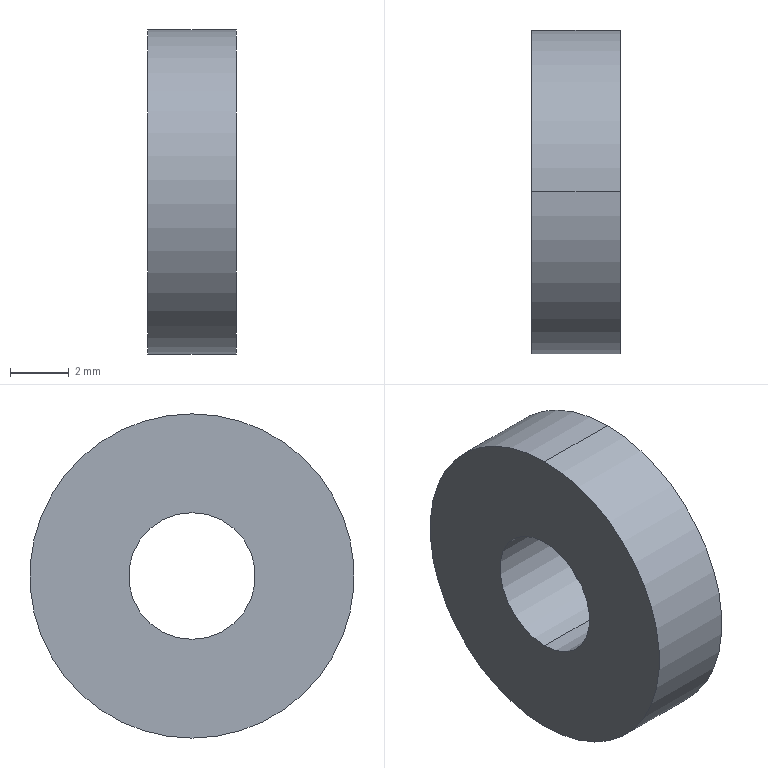Part | STEP file | 11-FJTM4_0_7_413part211 | 1 solid | 6 faces | box 3 x 11 x 11 mm | volume 241.533 mm3 | cylinder 4 | plane 2 | commonest cylinder face diameters 4.3 x2 11 x2
STEP:
#1=CARTESIAN_POINT('',(3.,0.,5.5));
#2=VERTEX_POINT('',#1);
#3=CARTESIAN_POINT('',(3.,0.,-5.5));
#4=VERTEX_POINT('',#3);
#5=CARTESIAN_POINT('',(3.,0.,0.));
#6=DIRECTION('',(-1.,0.,0.));
#7=DIRECTION('',(0.,0.,1.));
#8=AXIS2_PLACEMENT_3D('',#5,#6,#7);
#9=CIRCLE('',#8,5.5);
#10=EDGE_CURVE('',#2,#4,#9,.T.);
#11=ORIENTED_EDGE('',*,*,#10,.T.);
#12=CARTESIAN_POINT('',(0.,0.,-5.5));
#13=VERTEX_POINT('',#12);
#14=CARTESIAN_POINT('',(3.,0.,-5.5));
#15=DIRECTION('',(-1.,0.,0.));
#16=VECTOR('',#15,1000.);
#17=LINE('',#14,#16);
#18=EDGE_CURVE('',#4,#13,#17,.T.);
#19=ORIENTED_EDGE('',*,*,#18,.T.);
#20=CARTESIAN_POINT('',(0.,0.,5.5));
#21=VERTEX_POINT('',#20);
#22=CARTESIAN_POINT('',(0.,0.,0.));
#23=DIRECTION('',(-1.,0.,0.));
#24=DIRECTION('',(0.,0.,1.));
#25=AXIS2_PLACEMENT_3D('',#22,#23,#24);
#26=CIRCLE('',#25,5.5);
#27=EDGE_CURVE('',#21,#13,#26,.T.);
#28=ORIENTED_EDGE('',*,*,#27,.F.);
#29=CARTESIAN_POINT('',(3.,0.,5.5));
#30=DIRECTION('',(-1.,0.,0.));
#31=VECTOR('',#30,1000.);
#32=LINE('',#29,#31);
#33=EDGE_CURVE('',#2,#21,#32,.T.);
#34=ORIENTED_EDGE('',*,*,#33,.F.);
#35=EDGE_LOOP('',(#11,#19,#28,#34));
#36=FACE_OUTER_BOUND('',#35,.T.);
#37=CARTESIAN_POINT('',(3.,0.,0.));
#38=DIRECTION('',(-1.,0.,0.));
#39=DIRECTION('',(0.,0.,1.));
#40=AXIS2_PLACEMENT_3D('',#37,#38,#39);
#41=CYLINDRICAL_SURFACE('',#40,5.5);
#42=ADVANCED_FACE('',(#36),#41,.T.);
#43=CARTESIAN_POINT('',(3.,0.,-2.15));
#44=VERTEX_POINT('',#43);
#45=CARTESIAN_POINT('',(3.,0.,2.15));
#46=VERTEX_POINT('',#45);
#47=CARTESIAN_POINT('',(3.,0.,0.));
#48=DIRECTION('',(-1.,0.,0.));
#49=DIRECTION('',(0.,0.,1.));
#50=AXIS2_PLACEMENT_3D('',#47,#48,#49);
#51=CIRCLE('',#50,2.15);
#52=EDGE_CURVE('',#44,#46,#51,.T.);
#53=ORIENTED_EDGE('',*,*,#52,.F.);
#54=CARTESIAN_POINT('',(0.,0.,-2.15));
#55=VERTEX_POINT('',#54);
#56=CARTESIAN_POINT('',(3.,0.,-2.15));
#57=DIRECTION('',(-1.,0.,0.));
#58=VECTOR('',#57,1000.);
#59=LINE('',#56,#58);
#60=EDGE_CURVE('',#44,#55,#59,.T.);
#61=ORIENTED_EDGE('',*,*,#60,.T.);
#62=CARTESIAN_POINT('',(0.,0.,2.15));
#63=VERTEX_POINT('',#62);
#64=CARTESIAN_POINT('',(0.,0.,0.));
#65=DIRECTION('',(-1.,0.,0.));
#66=DIRECTION('',(0.,0.,1.));
#67=AXIS2_PLACEMENT_3D('',#64,#65,#66);
#68=CIRCLE('',#67,2.15);
#69=EDGE_CURVE('',#55,#63,#68,.T.);
#70=ORIENTED_EDGE('',*,*,#69,.T.);
#71=CARTESIAN_POINT('',(3.,0.,2.15));
#72=DIRECTION('',(-1.,0.,0.));
#73=VECTOR('',#72,1000.);
#74=LINE('',#71,#73);
#75=EDGE_CURVE('',#46,#63,#74,.T.);
#76=ORIENTED_EDGE('',*,*,#75,.F.);
#77=EDGE_LOOP('',(#53,#61,#70,#76));
#78=FACE_OUTER_BOUND('',#77,.T.);
#79=CARTESIAN_POINT('',(3.,0.,0.));
#80=DIRECTION('',(-1.,0.,0.));
#81=DIRECTION('',(0.,0.,1.));
#82=AXIS2_PLACEMENT_3D('',#79,#80,#81);
#83=CYLINDRICAL_SURFACE('',#82,2.15);
#84=ADVANCED_FACE('',(#78),#83,.F.);
#85=CARTESIAN_POINT('',(0.,0.,0.));
#86=DIRECTION('',(-1.,0.,0.));
#87=DIRECTION('',(0.,0.,1.));
#88=AXIS2_PLACEMENT_3D('',#85,#86,#87);
#89=CIRCLE('',#88,2.15);
#90=EDGE_CURVE('',#63,#55,#89,.T.);
#91=ORIENTED_EDGE('',*,*,#90,.F.);
#92=ORIENTED_EDGE('',*,*,#69,.F.);
#93=EDGE_LOOP('',(#91,#92));
#94=FACE_BOUND('',#93,.T.);
#95=ORIENTED_EDGE('',*,*,#27,.T.);
#96=CARTESIAN_POINT('',(0.,0.,0.));
#97=DIRECTION('',(-1.,0.,0.));
#98=DIRECTION('',(0.,0.,1.));
#99=AXIS2_PLACEMENT_3D('',#96,#97,#98);
#100=CIRCLE('',#99,5.5);
#101=EDGE_CURVE('',#13,#21,#100,.T.);
#102=ORIENTED_EDGE('',*,*,#101,.T.);
#103=EDGE_LOOP('',(#95,#102));
#104=FACE_OUTER_BOUND('',#103,.T.);
#105=CARTESIAN_POINT('',(0.,5.5,0.));
#106=DIRECTION('',(1.,0.,0.));
#107=DIRECTION('',(0.,0.,-1.));
#108=AXIS2_PLACEMENT_3D('',#105,#106,#107);
#109=PLANE('',#108);
#110=ADVANCED_FACE('',(#94,#104),#109,.F.);
#111=ORIENTED_EDGE('',*,*,#60,.F.);
#112=CARTESIAN_POINT('',(3.,0.,0.));
#113=DIRECTION('',(-1.,0.,0.));
#114=DIRECTION('',(0.,0.,1.));
#115=AXIS2_PLACEMENT_3D('',#112,#113,#114);
#116=CIRCLE('',#115,2.15);
#117=EDGE_CURVE('',#46,#44,#116,.T.);
#118=ORIENTED_EDGE('',*,*,#117,.F.);
#119=ORIENTED_EDGE('',*,*,#75,.T.);
#120=ORIENTED_EDGE('',*,*,#90,.T.);
#121=EDGE_LOOP('',(#111,#118,#119,#120));
#122=FACE_OUTER_BOUND('',#121,.T.);
#123=CARTESIAN_POINT('',(3.,0.,0.));
#124=DIRECTION('',(-1.,0.,0.));
#125=DIRECTION('',(0.,0.,1.));
#126=AXIS2_PLACEMENT_3D('',#123,#124,#125);
#127=CYLINDRICAL_SURFACE('',#126,2.15);
#128=ADVANCED_FACE('',(#122),#127,.F.);
#129=ORIENTED_EDGE('',*,*,#10,.F.);
#130=CARTESIAN_POINT('',(3.,0.,0.));
#131=DIRECTION('',(-1.,0.,0.));
#132=DIRECTION('',(0.,0.,1.));
#133=AXIS2_PLACEMENT_3D('',#130,#131,#132);
#134=CIRCLE('',#133,5.5);
#135=EDGE_CURVE('',#4,#2,#134,.T.);
#136=ORIENTED_EDGE('',*,*,#135,.F.);
#137=EDGE_LOOP('',(#129,#136));
#138=FACE_OUTER_BOUND('',#137,.T.);
#139=ORIENTED_EDGE('',*,*,#117,.T.);
#140=ORIENTED_EDGE('',*,*,#52,.T.);
#141=EDGE_LOOP('',(#139,#140));
#142=FACE_BOUND('',#141,.T.);
#143=CARTESIAN_POINT('',(3.,2.15,0.));
#144=DIRECTION('',(-1.,0.,0.));
#145=DIRECTION('',(0.,0.,1.));
#146=AXIS2_PLACEMENT_3D('',#143,#144,#145);
#147=PLANE('',#146);
#148=ADVANCED_FACE('',(#138,#142),#147,.F.);
#149=ORIENTED_EDGE('',*,*,#18,.F.);
#150=ORIENTED_EDGE('',*,*,#135,.T.);
#151=ORIENTED_EDGE('',*,*,#33,.T.);
#152=ORIENTED_EDGE('',*,*,#101,.F.);
#153=EDGE_LOOP('',(#149,#150,#151,#152));
#154=FACE_OUTER_BOUND('',#153,.T.);
#155=CARTESIAN_POINT('',(3.,0.,0.));
#156=DIRECTION('',(-1.,0.,0.));
#157=DIRECTION('',(0.,0.,1.));
#158=AXIS2_PLACEMENT_3D('',#155,#156,#157);
#159=CYLINDRICAL_SURFACE('',#158,5.5);
#160=ADVANCED_FACE('',(#154),#159,.T.);
#161=CLOSED_SHELL('',(#42,#84,#110,#128,#148,#160));
#162=MANIFOLD_SOLID_BREP('',#161);
#163=CARTESIAN_POINT('',(0.,0.,0.));
#164=DIRECTION('',(0.,0.,1.));
#165=DIRECTION('',(1.,0.,0.));
#166=AXIS2_PLACEMENT_3D('',#163,#164,#165);
#167=(LENGTH_UNIT()NAMED_UNIT(*)SI_UNIT(.MILLI.,.METRE.));
#168=UNCERTAINTY_MEASURE_WITH_UNIT(LENGTH_MEASURE(0.00001),#167,'','');
#169=(NAMED_UNIT(*)PLANE_ANGLE_UNIT()SI_UNIT($,.RADIAN.));
#170=(NAMED_UNIT(*)SI_UNIT($,.STERADIAN.)SOLID_ANGLE_UNIT());
#171=(GEOMETRIC_REPRESENTATION_CONTEXT(3)GLOBAL_UNCERTAINTY_ASSIGNED_CONTEXT((#168))GLOBAL_UNIT_ASSIGNED_CONTEXT((#167,#169,#170))REPRESENTATION_CONTEXT('',''));
#172=ADVANCED_BREP_SHAPE_REPRESENTATION('',(#162,#166),#171);